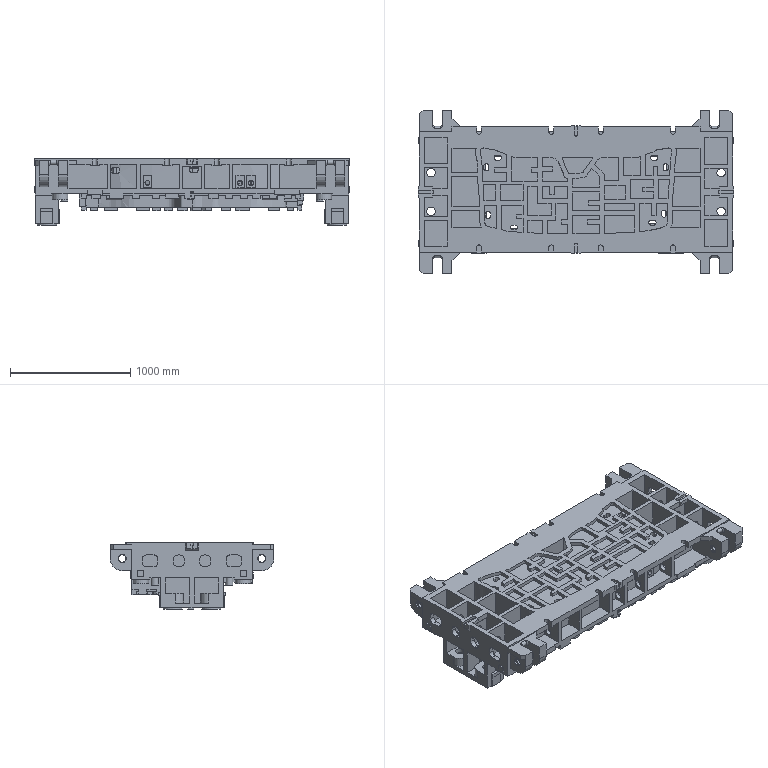Part | NX | features solid 2 | 1 solid | 1720 faces | box 2620 x 1360 x 550 mm | volume 362567696 mm3 | plane 1373 | cylinder 294 | spline 42 | torus 8 | cone 3 | commonest cylinder face diameters 80 x58 68 x48 60 x47 40 x44 30 x16 64 x16